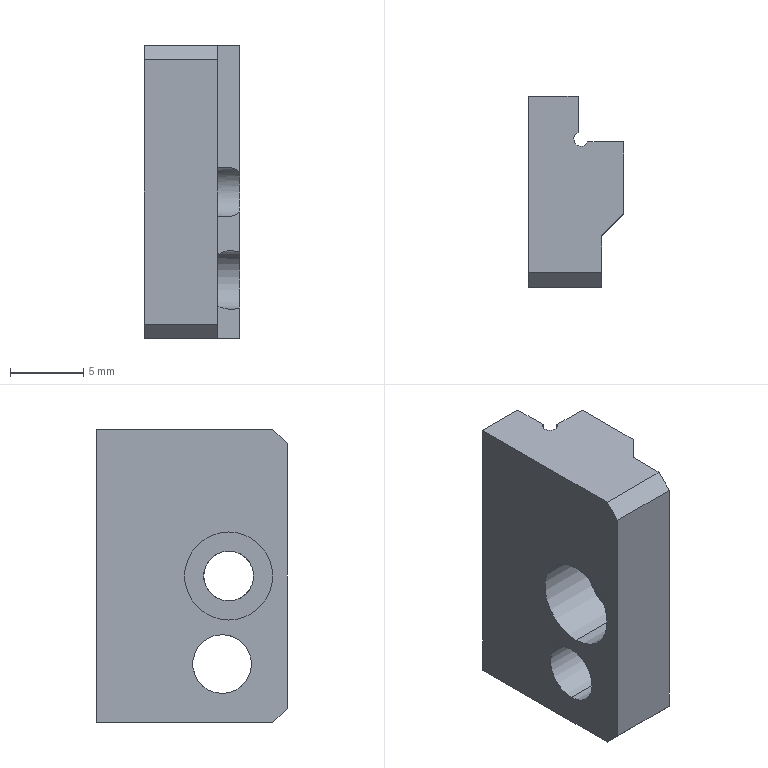Part | SolidWorks | features Cut 2, Chamfer 1, Extrusion 1, HoleWzd 1 | 1 solid | 23 faces | box 6.5 x 13 x 20 mm | volume 1157 mm3 | plane 15 | cylinder 8 | commonest cylinder face diameters 1 x2 3.4 x2 4 x2 6 x2
STEP:
#1=CARTESIAN_POINT('',(5.95,4.45,2.));
#2=VERTEX_POINT('',#1);
#3=CARTESIAN_POINT('',(5.,3.5,2.24));
#4=VERTEX_POINT('',#3);
#5=CARTESIAN_POINT('',(5.95,4.45,2.));
#6=CARTESIAN_POINT('',(5.617,4.117,2.));
#7=CARTESIAN_POINT('',(5.293,3.793,2.082));
#8=CARTESIAN_POINT('',(5.,3.5,2.24));
#9=(BOUNDED_CURVE()B_SPLINE_CURVE(3,(#5,#6,#7,#8),.UNSPECIFIED.,.F.,.F.)B_SPLINE_CURVE_WITH_KNOTS((4,4),(4.712,5.207),.UNSPECIFIED.)CURVE()GEOMETRIC_REPRESENTATION_ITEM()RATIONAL_B_SPLINE_CURVE((1.,0.9797,0.9797,1.))REPRESENTATION_ITEM(''));
#10=EDGE_CURVE('',#2,#4,#9,.T.);
#11=ORIENTED_EDGE('',*,*,#10,.F.);
#12=CARTESIAN_POINT('',(0.,4.45,2.));
#13=VERTEX_POINT('',#12);
#14=CARTESIAN_POINT('',(8.,4.45,2.));
#15=DIRECTION('',(-1.,0.,0.));
#16=VECTOR('',#15,1000.);
#17=LINE('',#14,#16);
#18=EDGE_CURVE('',#2,#13,#17,.T.);
#19=ORIENTED_EDGE('',*,*,#18,.T.);
#20=CARTESIAN_POINT('',(0.,4.45,6.));
#21=VERTEX_POINT('',#20);
#22=CARTESIAN_POINT('',(0.,4.45,4.));
#23=DIRECTION('',(-1.,0.,0.));
#24=DIRECTION('',(0.,0.,1.));
#25=AXIS2_PLACEMENT_3D('',#22,#23,#24);
#26=CIRCLE('',#25,2.);
#27=EDGE_CURVE('',#13,#21,#26,.T.);
#28=ORIENTED_EDGE('',*,*,#27,.T.);
#29=CARTESIAN_POINT('',(5.95,4.45,6.));
#30=VERTEX_POINT('',#29);
#31=CARTESIAN_POINT('',(8.,4.45,6.));
#32=DIRECTION('',(-1.,0.,0.));
#33=VECTOR('',#32,1000.);
#34=LINE('',#31,#33);
#35=EDGE_CURVE('',#30,#21,#34,.T.);
#36=ORIENTED_EDGE('',*,*,#35,.F.);
#37=CARTESIAN_POINT('',(5.,3.5,5.76));
#38=VERTEX_POINT('',#37);
#39=CARTESIAN_POINT('',(5.,3.5,5.76));
#40=CARTESIAN_POINT('',(5.293,3.793,5.918));
#41=CARTESIAN_POINT('',(5.617,4.117,6.));
#42=CARTESIAN_POINT('',(5.95,4.45,6.));
#43=(BOUNDED_CURVE()B_SPLINE_CURVE(3,(#39,#40,#41,#42),.UNSPECIFIED.,.F.,.T.)B_SPLINE_CURVE_WITH_KNOTS((4,4),(1.076,1.571),.UNSPECIFIED.)CURVE()GEOMETRIC_REPRESENTATION_ITEM()RATIONAL_B_SPLINE_CURVE((1.,0.9797,0.9797,1.))REPRESENTATION_ITEM(''));
#44=EDGE_CURVE('',#38,#30,#43,.T.);
#45=ORIENTED_EDGE('',*,*,#44,.F.);
#46=CARTESIAN_POINT('',(5.,4.45,4.));
#47=DIRECTION('',(-1.,0.,0.));
#48=DIRECTION('',(0.,0.,1.));
#49=AXIS2_PLACEMENT_3D('',#46,#47,#48);
#50=CIRCLE('',#49,2.);
#51=EDGE_CURVE('',#4,#38,#50,.T.);
#52=ORIENTED_EDGE('',*,*,#51,.F.);
#53=EDGE_LOOP('',(#11,#19,#28,#36,#45,#52));
#54=FACE_OUTER_BOUND('',#53,.T.);
#55=CARTESIAN_POINT('',(8.,4.45,4.));
#56=DIRECTION('',(-1.,0.,0.));
#57=DIRECTION('',(0.,0.,1.));
#58=AXIS2_PLACEMENT_3D('',#55,#56,#57);
#59=CYLINDRICAL_SURFACE('',#58,2.);
#60=ADVANCED_FACE('',(#54),#59,.F.);
#61=CARTESIAN_POINT('',(4.,4.,7.));
#62=VERTEX_POINT('',#61);
#63=CARTESIAN_POINT('',(4.,4.,13.));
#64=VERTEX_POINT('',#63);
#65=CARTESIAN_POINT('',(4.,4.,10.));
#66=DIRECTION('',(-1.,0.,0.));
#67=DIRECTION('',(0.,0.,1.));
#68=AXIS2_PLACEMENT_3D('',#65,#66,#67);
#69=CIRCLE('',#68,3.);
#70=EDGE_CURVE('',#62,#64,#69,.T.);
#71=ORIENTED_EDGE('',*,*,#70,.F.);
#72=CARTESIAN_POINT('',(0.,4.,7.));
#73=VERTEX_POINT('',#72);
#74=CARTESIAN_POINT('',(0.,4.,7.));
#75=DIRECTION('',(-1.,0.,0.));
#76=VECTOR('',#75,1000.);
#77=LINE('',#74,#76);
#78=EDGE_CURVE('',#62,#73,#77,.T.);
#79=ORIENTED_EDGE('',*,*,#78,.T.);
#80=CARTESIAN_POINT('',(0.,4.,13.));
#81=VERTEX_POINT('',#80);
#82=CARTESIAN_POINT('',(0.,4.,10.));
#83=DIRECTION('',(-1.,0.,0.));
#84=DIRECTION('',(0.,0.,1.));
#85=AXIS2_PLACEMENT_3D('',#82,#83,#84);
#86=CIRCLE('',#85,3.);
#87=EDGE_CURVE('',#73,#81,#86,.T.);
#88=ORIENTED_EDGE('',*,*,#87,.T.);
#89=CARTESIAN_POINT('',(0.,4.,13.));
#90=DIRECTION('',(-1.,0.,0.));
#91=VECTOR('',#90,1000.);
#92=LINE('',#89,#91);
#93=EDGE_CURVE('',#64,#81,#92,.T.);
#94=ORIENTED_EDGE('',*,*,#93,.F.);
#95=EDGE_LOOP('',(#71,#79,#88,#94));
#96=FACE_OUTER_BOUND('',#95,.T.);
#97=CARTESIAN_POINT('',(0.,4.,10.));
#98=DIRECTION('',(-1.,0.,0.));
#99=DIRECTION('',(0.,0.,1.));
#100=AXIS2_PLACEMENT_3D('',#97,#98,#99);
#101=CYLINDRICAL_SURFACE('',#100,3.);
#102=ADVANCED_FACE('',(#96),#101,.F.);
#103=CARTESIAN_POINT('',(5.5,4.,8.3));
#104=VERTEX_POINT('',#103);
#105=CARTESIAN_POINT('',(5.,3.5,8.375));
#106=VERTEX_POINT('',#105);
#107=CARTESIAN_POINT('',(5.5,4.,8.3));
#108=CARTESIAN_POINT('',(5.33,3.83,8.3));
#109=CARTESIAN_POINT('',(5.162,3.662,8.325));
#110=CARTESIAN_POINT('',(5.,3.5,8.375));
#111=(BOUNDED_CURVE()B_SPLINE_CURVE(3,(#107,#108,#109,#110),.UNSPECIFIED.,.F.,.F.)B_SPLINE_CURVE_WITH_KNOTS((4,4),(4.712,5.011),.UNSPECIFIED.)CURVE()GEOMETRIC_REPRESENTATION_ITEM()RATIONAL_B_SPLINE_CURVE((1.,0.9926,0.9926,1.))REPRESENTATION_ITEM(''));
#112=EDGE_CURVE('',#104,#106,#111,.T.);
#113=ORIENTED_EDGE('',*,*,#112,.F.);
#114=CARTESIAN_POINT('',(4.,4.,8.3));
#115=VERTEX_POINT('',#114);
#116=CARTESIAN_POINT('',(0.,4.,8.3));
#117=DIRECTION('',(-1.,0.,0.));
#118=VECTOR('',#117,1000.);
#119=LINE('',#116,#118);
#120=EDGE_CURVE('',#104,#115,#119,.T.);
#121=ORIENTED_EDGE('',*,*,#120,.T.);
#122=CARTESIAN_POINT('',(4.,4.,11.7));
#123=VERTEX_POINT('',#122);
#124=CARTESIAN_POINT('',(4.,4.,10.));
#125=DIRECTION('',(-1.,0.,0.));
#126=DIRECTION('',(0.,0.,1.));
#127=AXIS2_PLACEMENT_3D('',#124,#125,#126);
#128=CIRCLE('',#127,1.7);
#129=EDGE_CURVE('',#115,#123,#128,.T.);
#130=ORIENTED_EDGE('',*,*,#129,.T.);
#131=CARTESIAN_POINT('',(5.5,4.,11.7));
#132=VERTEX_POINT('',#131);
#133=CARTESIAN_POINT('',(0.,4.,11.7));
#134=DIRECTION('',(-1.,0.,0.));
#135=VECTOR('',#134,1000.);
#136=LINE('',#133,#135);
#137=EDGE_CURVE('',#132,#123,#136,.T.);
#138=ORIENTED_EDGE('',*,*,#137,.F.);
#139=CARTESIAN_POINT('',(5.,3.5,11.625));
#140=VERTEX_POINT('',#139);
#141=CARTESIAN_POINT('',(5.,3.5,11.625));
#142=CARTESIAN_POINT('',(5.162,3.662,11.675));
#143=CARTESIAN_POINT('',(5.33,3.83,11.7));
#144=CARTESIAN_POINT('',(5.5,4.,11.7));
#145=(BOUNDED_CURVE()B_SPLINE_CURVE(3,(#141,#142,#143,#144),.UNSPECIFIED.,.F.,.F.)B_SPLINE_CURVE_WITH_KNOTS((4,4),(1.272,1.571),.UNSPECIFIED.)CURVE()GEOMETRIC_REPRESENTATION_ITEM()RATIONAL_B_SPLINE_CURVE((1.,0.9926,0.9926,1.))REPRESENTATION_ITEM(''));
#146=EDGE_CURVE('',#140,#132,#145,.T.);
#147=ORIENTED_EDGE('',*,*,#146,.F.);
#148=CARTESIAN_POINT('',(5.,4.,10.));
#149=DIRECTION('',(-1.,0.,0.));
#150=DIRECTION('',(0.,0.,1.));
#151=AXIS2_PLACEMENT_3D('',#148,#149,#150);
#152=CIRCLE('',#151,1.7);
#153=EDGE_CURVE('',#106,#140,#152,.T.);
#154=ORIENTED_EDGE('',*,*,#153,.F.);
#155=EDGE_LOOP('',(#113,#121,#130,#138,#147,#154));
#156=FACE_OUTER_BOUND('',#155,.T.);
#157=CARTESIAN_POINT('',(0.,4.,10.));
#158=DIRECTION('',(-1.,0.,0.));
#159=DIRECTION('',(0.,0.,1.));
#160=AXIS2_PLACEMENT_3D('',#157,#158,#159);
#161=CYLINDRICAL_SURFACE('',#160,1.7);
#162=ADVANCED_FACE('',(#156),#161,.F.);
#163=CARTESIAN_POINT('',(3.1,10.1,20.));
#164=VERTEX_POINT('',#163);
#165=CARTESIAN_POINT('',(3.4,10.558,20.));
#166=VERTEX_POINT('',#165);
#167=CARTESIAN_POINT('',(3.6,10.1,20.));
#168=DIRECTION('',(0.,0.,-1.));
#169=DIRECTION('',(1.,0.,0.));
#170=AXIS2_PLACEMENT_3D('',#167,#168,#169);
#171=CIRCLE('',#170,0.5);
#172=EDGE_CURVE('',#164,#166,#171,.T.);
#173=ORIENTED_EDGE('',*,*,#172,.F.);
#174=CARTESIAN_POINT('',(3.1,10.1,0.));
#175=VERTEX_POINT('',#174);
#176=CARTESIAN_POINT('',(3.1,10.1,20.));
#177=DIRECTION('',(0.,0.,-1.));
#178=VECTOR('',#177,1000.);
#179=LINE('',#176,#178);
#180=EDGE_CURVE('',#164,#175,#179,.T.);
#181=ORIENTED_EDGE('',*,*,#180,.T.);
#182=CARTESIAN_POINT('',(3.4,10.558,0.));
#183=VERTEX_POINT('',#182);
#184=CARTESIAN_POINT('',(3.6,10.1,0.));
#185=DIRECTION('',(0.,0.,-1.));
#186=DIRECTION('',(1.,0.,0.));
#187=AXIS2_PLACEMENT_3D('',#184,#185,#186);
#188=CIRCLE('',#187,0.5);
#189=EDGE_CURVE('',#175,#183,#188,.T.);
#190=ORIENTED_EDGE('',*,*,#189,.T.);
#191=CARTESIAN_POINT('',(3.4,10.558,20.));
#192=DIRECTION('',(0.,0.,-1.));
#193=VECTOR('',#192,1000.);
#194=LINE('',#191,#193);
#195=EDGE_CURVE('',#166,#183,#194,.T.);
#196=ORIENTED_EDGE('',*,*,#195,.F.);
#197=EDGE_LOOP('',(#173,#181,#190,#196));
#198=FACE_OUTER_BOUND('',#197,.T.);
#199=CARTESIAN_POINT('',(3.6,10.1,20.));
#200=DIRECTION('',(0.,0.,-1.));
#201=DIRECTION('',(-1.,0.,0.));
#202=AXIS2_PLACEMENT_3D('',#199,#200,#201);
#203=CYLINDRICAL_SURFACE('',#202,0.5);
#204=ADVANCED_FACE('',(#198),#203,.F.);
#205=CARTESIAN_POINT('',(5.,3.5,-5.22));
#206=DIRECTION('',(0.,0.,1.));
#207=VECTOR('',#206,1000.);
#208=LINE('',#205,#207);
#209=EDGE_CURVE('',#38,#106,#208,.T.);
#210=ORIENTED_EDGE('',*,*,#209,.F.);
#211=ORIENTED_EDGE('',*,*,#44,.T.);
#212=CARTESIAN_POINT('',(6.5,5.,5.923));
#213=VERTEX_POINT('',#212);
#214=CARTESIAN_POINT('',(5.95,4.45,6.));
#215=CARTESIAN_POINT('',(6.136,4.636,6.));
#216=CARTESIAN_POINT('',(6.321,4.821,5.974));
#217=CARTESIAN_POINT('',(6.5,5.,5.923));
#218=(BOUNDED_CURVE()B_SPLINE_CURVE(3,(#214,#215,#216,#217),.UNSPECIFIED.,.F.,.F.)B_SPLINE_CURVE_WITH_KNOTS((4,4),(1.571,1.849),.UNSPECIFIED.)CURVE()GEOMETRIC_REPRESENTATION_ITEM()RATIONAL_B_SPLINE_CURVE((1.,0.9935,0.9935,1.))REPRESENTATION_ITEM(''));
#219=EDGE_CURVE('',#30,#213,#218,.T.);
#220=ORIENTED_EDGE('',*,*,#219,.T.);
#221=CARTESIAN_POINT('',(6.5,5.,8.625));
#222=VERTEX_POINT('',#221);
#223=CARTESIAN_POINT('',(6.5,5.,-5.22));
#224=DIRECTION('',(0.,0.,1.));
#225=VECTOR('',#224,1000.);
#226=LINE('',#223,#225);
#227=EDGE_CURVE('',#213,#222,#226,.T.);
#228=ORIENTED_EDGE('',*,*,#227,.T.);
#229=CARTESIAN_POINT('',(6.5,5.,8.625));
#230=CARTESIAN_POINT('',(6.207,4.707,8.412));
#231=CARTESIAN_POINT('',(5.862,4.362,8.3));
#232=CARTESIAN_POINT('',(5.5,4.,8.3));
#233=(BOUNDED_CURVE()B_SPLINE_CURVE(3,(#229,#230,#231,#232),.UNSPECIFIED.,.F.,.F.)B_SPLINE_CURVE_WITH_KNOTS((4,4),(4.084,4.712),.UNSPECIFIED.)CURVE()GEOMETRIC_REPRESENTATION_ITEM()RATIONAL_B_SPLINE_CURVE((1.,0.9673,0.9673,1.))REPRESENTATION_ITEM(''));
#234=EDGE_CURVE('',#222,#104,#233,.T.);
#235=ORIENTED_EDGE('',*,*,#234,.T.);
#236=ORIENTED_EDGE('',*,*,#112,.T.);
#237=EDGE_LOOP('',(#210,#211,#220,#228,#235,#236));
#238=FACE_OUTER_BOUND('',#237,.T.);
#239=CARTESIAN_POINT('',(6.5,5.,-5.22));
#240=DIRECTION('',(-0.7071,0.7071,0.));
#241=DIRECTION('',(-0.7071,-0.7071,0.));
#242=AXIS2_PLACEMENT_3D('',#239,#240,#241);
#243=PLANE('',#242);
#244=ADVANCED_FACE('',(#238),#243,.F.);
#245=CARTESIAN_POINT('',(5.,3.5,20.));
#246=VERTEX_POINT('',#245);
#247=CARTESIAN_POINT('',(5.,3.5,-5.22));
#248=DIRECTION('',(0.,0.,1.));
#249=VECTOR('',#248,1000.);
#250=LINE('',#247,#249);
#251=EDGE_CURVE('',#140,#246,#250,.T.);
#252=ORIENTED_EDGE('',*,*,#251,.F.);
#253=ORIENTED_EDGE('',*,*,#146,.T.);
#254=CARTESIAN_POINT('',(6.5,5.,11.375));
#255=VERTEX_POINT('',#254);
#256=CARTESIAN_POINT('',(5.5,4.,11.7));
#257=CARTESIAN_POINT('',(5.862,4.362,11.7));
#258=CARTESIAN_POINT('',(6.207,4.707,11.588));
#259=CARTESIAN_POINT('',(6.5,5.,11.375));
#260=(BOUNDED_CURVE()B_SPLINE_CURVE(3,(#256,#257,#258,#259),.UNSPECIFIED.,.F.,.F.)B_SPLINE_CURVE_WITH_KNOTS((4,4),(1.571,2.2),.UNSPECIFIED.)CURVE()GEOMETRIC_REPRESENTATION_ITEM()RATIONAL_B_SPLINE_CURVE((1.,0.9673,0.9673,1.))REPRESENTATION_ITEM(''));
#261=EDGE_CURVE('',#132,#255,#260,.T.);
#262=ORIENTED_EDGE('',*,*,#261,.T.);
#263=CARTESIAN_POINT('',(6.5,5.,20.));
#264=VERTEX_POINT('',#263);
#265=CARTESIAN_POINT('',(6.5,5.,-5.22));
#266=DIRECTION('',(0.,0.,1.));
#267=VECTOR('',#266,1000.);
#268=LINE('',#265,#267);
#269=EDGE_CURVE('',#255,#264,#268,.T.);
#270=ORIENTED_EDGE('',*,*,#269,.T.);
#271=CARTESIAN_POINT('',(6.5,5.,20.));
#272=DIRECTION('',(-0.7071,-0.7071,0.));
#273=VECTOR('',#272,1000.);
#274=LINE('',#271,#273);
#275=EDGE_CURVE('',#264,#246,#274,.T.);
#276=ORIENTED_EDGE('',*,*,#275,.T.);
#277=EDGE_LOOP('',(#252,#253,#262,#270,#276));
#278=FACE_OUTER_BOUND('',#277,.T.);
#279=CARTESIAN_POINT('',(6.5,5.,-5.22));
#280=DIRECTION('',(-0.7071,0.7071,0.));
#281=DIRECTION('',(-0.7071,-0.7071,0.));
#282=AXIS2_PLACEMENT_3D('',#279,#280,#281);
#283=PLANE('',#282);
#284=ADVANCED_FACE('',(#278),#283,.F.);
#285=CARTESIAN_POINT('',(5.,0.,1.));
#286=VERTEX_POINT('',#285);
#287=CARTESIAN_POINT('',(5.,0.,19.));
#288=VERTEX_POINT('',#287);
#289=CARTESIAN_POINT('',(5.,0.,-5.22));
#290=DIRECTION('',(0.,0.,1.));
#291=VECTOR('',#290,1000.);
#292=LINE('',#289,#291);
#293=EDGE_CURVE('',#286,#288,#292,.T.);
#294=ORIENTED_EDGE('',*,*,#293,.T.);
#295=CARTESIAN_POINT('',(0.,0.,19.));
#296=VERTEX_POINT('',#295);
#297=CARTESIAN_POINT('',(0.,0.,19.));
#298=DIRECTION('',(-1.,0.,0.));
#299=VECTOR('',#298,1000.);
#300=LINE('',#297,#299);
#301=EDGE_CURVE('',#288,#296,#300,.T.);
#302=ORIENTED_EDGE('',*,*,#301,.T.);
#303=CARTESIAN_POINT('',(0.,0.,1.));
#304=VERTEX_POINT('',#303);
#305=CARTESIAN_POINT('',(0.,0.,20.));
#306=DIRECTION('',(0.,0.,-1.));
#307=VECTOR('',#306,1000.);
#308=LINE('',#305,#307);
#309=EDGE_CURVE('',#296,#304,#308,.T.);
#310=ORIENTED_EDGE('',*,*,#309,.T.);
#311=CARTESIAN_POINT('',(6.5,0.,1.));
#312=DIRECTION('',(1.,0.,0.));
#313=VECTOR('',#312,1000.);
#314=LINE('',#311,#313);
#315=EDGE_CURVE('',#304,#286,#314,.T.);
#316=ORIENTED_EDGE('',*,*,#315,.T.);
#317=EDGE_LOOP('',(#294,#302,#310,#316));
#318=FACE_OUTER_BOUND('',#317,.T.);
#319=CARTESIAN_POINT('',(6.5,0.,20.));
#320=DIRECTION('',(0.,1.,0.));
#321=DIRECTION('',(-1.,0.,0.));
#322=AXIS2_PLACEMENT_3D('',#319,#320,#321);
#323=PLANE('',#322);
#324=ADVANCED_FACE('',(#318),#323,.F.);
#325=ORIENTED_EDGE('',*,*,#227,.F.);
#326=CARTESIAN_POINT('',(6.5,5.,2.077));
#327=VERTEX_POINT('',#326);
#328=CARTESIAN_POINT('',(6.5,4.45,4.));
#329=DIRECTION('',(-1.,0.,0.));
#330=DIRECTION('',(0.,-1.,0.));
#331=AXIS2_PLACEMENT_3D('',#328,#329,#330);
#332=CIRCLE('',#331,2.);
#333=EDGE_CURVE('',#213,#327,#332,.T.);
#334=ORIENTED_EDGE('',*,*,#333,.T.);
#335=CARTESIAN_POINT('',(6.5,5.,0.));
#336=VERTEX_POINT('',#335);
#337=CARTESIAN_POINT('',(6.5,5.,-5.22));
#338=DIRECTION('',(0.,0.,1.));
#339=VECTOR('',#338,1000.);
#340=LINE('',#337,#339);
#341=EDGE_CURVE('',#336,#327,#340,.T.);
#342=ORIENTED_EDGE('',*,*,#341,.F.);
#343=CARTESIAN_POINT('',(6.5,9.9,0.));
#344=VERTEX_POINT('',#343);
#345=CARTESIAN_POINT('',(6.5,9.9,0.));
#346=DIRECTION('',(0.,1.,0.));
#347=VECTOR('',#346,1000.);
#348=LINE('',#345,#347);
#349=EDGE_CURVE('',#336,#344,#348,.T.);
#350=ORIENTED_EDGE('',*,*,#349,.T.);
#351=CARTESIAN_POINT('',(6.5,9.9,20.));
#352=VERTEX_POINT('',#351);
#353=CARTESIAN_POINT('',(6.5,9.9,20.));
#354=DIRECTION('',(0.,0.,-1.));
#355=VECTOR('',#354,1000.);
#356=LINE('',#353,#355);
#357=EDGE_CURVE('',#352,#344,#356,.T.);
#358=ORIENTED_EDGE('',*,*,#357,.F.);
#359=CARTESIAN_POINT('',(6.5,9.9,20.));
#360=DIRECTION('',(0.,1.,0.));
#361=VECTOR('',#360,1000.);
#362=LINE('',#359,#361);
#363=EDGE_CURVE('',#264,#352,#362,.T.);
#364=ORIENTED_EDGE('',*,*,#363,.F.);
#365=ORIENTED_EDGE('',*,*,#269,.F.);
#366=CARTESIAN_POINT('',(6.5,4.,10.));
#367=DIRECTION('',(-1.,0.,0.));
#368=DIRECTION('',(0.,-1.,0.));
#369=AXIS2_PLACEMENT_3D('',#366,#367,#368);
#370=CIRCLE('',#369,1.7);
#371=EDGE_CURVE('',#255,#222,#370,.T.);
#372=ORIENTED_EDGE('',*,*,#371,.T.);
#373=EDGE_LOOP('',(#325,#334,#342,#350,#358,#364,#365,#372));
#374=FACE_OUTER_BOUND('',#373,.T.);
#375=CARTESIAN_POINT('',(6.5,9.9,20.));
#376=DIRECTION('',(-1.,0.,0.));
#377=DIRECTION('',(0.,-1.,0.));
#378=AXIS2_PLACEMENT_3D('',#375,#376,#377);
#379=PLANE('',#378);
#380=ADVANCED_FACE('',(#374),#379,.F.);
#381=CARTESIAN_POINT('',(4.058,9.9,0.));
#382=VERTEX_POINT('',#381);
#383=CARTESIAN_POINT('',(4.058,9.9,0.));
#384=DIRECTION('',(-1.,0.,0.));
#385=VECTOR('',#384,1000.);
#386=LINE('',#383,#385);
#387=EDGE_CURVE('',#344,#382,#386,.T.);
#388=ORIENTED_EDGE('',*,*,#387,.T.);
#389=CARTESIAN_POINT('',(4.058,9.9,20.));
#390=VERTEX_POINT('',#389);
#391=CARTESIAN_POINT('',(4.058,9.9,20.));
#392=DIRECTION('',(0.,0.,-1.));
#393=VECTOR('',#392,1000.);
#394=LINE('',#391,#393);
#395=EDGE_CURVE('',#390,#382,#394,.T.);
#396=ORIENTED_EDGE('',*,*,#395,.F.);
#397=CARTESIAN_POINT('',(4.058,9.9,20.));
#398=DIRECTION('',(-1.,0.,0.));
#399=VECTOR('',#398,1000.);
#400=LINE('',#397,#399);
#401=EDGE_CURVE('',#352,#390,#400,.T.);
#402=ORIENTED_EDGE('',*,*,#401,.F.);
#403=ORIENTED_EDGE('',*,*,#357,.T.);
#404=EDGE_LOOP('',(#388,#396,#402,#403));
#405=FACE_OUTER_BOUND('',#404,.T.);
#406=CARTESIAN_POINT('',(4.058,9.9,20.));
#407=DIRECTION('',(0.,-1.,0.));
#408=DIRECTION('',(1.,0.,0.));
#409=AXIS2_PLACEMENT_3D('',#406,#407,#408);
#410=PLANE('',#409);
#411=ADVANCED_FACE('',(#405),#410,.F.);
#412=ORIENTED_EDGE('',*,*,#180,.F.);
#413=CARTESIAN_POINT('',(3.6,10.1,20.));
#414=DIRECTION('',(0.,0.,-1.));
#415=DIRECTION('',(1.,0.,0.));
#416=AXIS2_PLACEMENT_3D('',#413,#414,#415);
#417=CIRCLE('',#416,0.5);
#418=EDGE_CURVE('',#390,#164,#417,.T.);
#419=ORIENTED_EDGE('',*,*,#418,.F.);
#420=ORIENTED_EDGE('',*,*,#395,.T.);
#421=CARTESIAN_POINT('',(3.6,10.1,0.));
#422=DIRECTION('',(0.,0.,-1.));
#423=DIRECTION('',(1.,0.,0.));
#424=AXIS2_PLACEMENT_3D('',#421,#422,#423);
#425=CIRCLE('',#424,0.5);
#426=EDGE_CURVE('',#382,#175,#425,.T.);
#427=ORIENTED_EDGE('',*,*,#426,.T.);
#428=EDGE_LOOP('',(#412,#419,#420,#427));
#429=FACE_OUTER_BOUND('',#428,.T.);
#430=CARTESIAN_POINT('',(3.6,10.1,20.));
#431=DIRECTION('',(0.,0.,-1.));
#432=DIRECTION('',(-1.,0.,0.));
#433=AXIS2_PLACEMENT_3D('',#430,#431,#432);
#434=CYLINDRICAL_SURFACE('',#433,0.5);
#435=ADVANCED_FACE('',(#429),#434,.F.);
#436=CARTESIAN_POINT('',(3.4,13.,0.));
#437=VERTEX_POINT('',#436);
#438=CARTESIAN_POINT('',(3.4,13.,0.));
#439=DIRECTION('',(0.,1.,0.));
#440=VECTOR('',#439,1000.);
#441=LINE('',#438,#440);
#442=EDGE_CURVE('',#183,#437,#441,.T.);
#443=ORIENTED_EDGE('',*,*,#442,.T.);
#444=CARTESIAN_POINT('',(3.4,13.,20.));
#445=VERTEX_POINT('',#444);
#446=CARTESIAN_POINT('',(3.4,13.,20.));
#447=DIRECTION('',(0.,0.,-1.));
#448=VECTOR('',#447,1000.);
#449=LINE('',#446,#448);
#450=EDGE_CURVE('',#445,#437,#449,.T.);
#451=ORIENTED_EDGE('',*,*,#450,.F.);
#452=CARTESIAN_POINT('',(3.4,13.,20.));
#453=DIRECTION('',(0.,1.,0.));
#454=VECTOR('',#453,1000.);
#455=LINE('',#452,#454);
#456=EDGE_CURVE('',#166,#445,#455,.T.);
#457=ORIENTED_EDGE('',*,*,#456,.F.);
#458=ORIENTED_EDGE('',*,*,#195,.T.);
#459=EDGE_LOOP('',(#443,#451,#457,#458));
#460=FACE_OUTER_BOUND('',#459,.T.);
#461=CARTESIAN_POINT('',(3.4,13.,20.));
#462=DIRECTION('',(-1.,0.,0.));
#463=DIRECTION('',(0.,-1.,0.));
#464=AXIS2_PLACEMENT_3D('',#461,#462,#463);
#465=PLANE('',#464);
#466=ADVANCED_FACE('',(#460),#465,.F.);
#467=CARTESIAN_POINT('',(0.,13.,0.));
#468=VERTEX_POINT('',#467);
#469=CARTESIAN_POINT('',(0.,13.,0.));
#470=DIRECTION('',(-1.,0.,0.));
#471=VECTOR('',#470,1000.);
#472=LINE('',#469,#471);
#473=EDGE_CURVE('',#437,#468,#472,.T.);
#474=ORIENTED_EDGE('',*,*,#473,.T.);
#475=CARTESIAN_POINT('',(0.,13.,20.));
#476=VERTEX_POINT('',#475);
#477=CARTESIAN_POINT('',(0.,13.,20.));
#478=DIRECTION('',(0.,0.,-1.));
#479=VECTOR('',#478,1000.);
#480=LINE('',#477,#479);
#481=EDGE_CURVE('',#476,#468,#480,.T.);
#482=ORIENTED_EDGE('',*,*,#481,.F.);
#483=CARTESIAN_POINT('',(0.,13.,20.));
#484=DIRECTION('',(-1.,0.,0.));
#485=VECTOR('',#484,1000.);
#486=LINE('',#483,#485);
#487=EDGE_CURVE('',#445,#476,#486,.T.);
#488=ORIENTED_EDGE('',*,*,#487,.F.);
#489=ORIENTED_EDGE('',*,*,#450,.T.);
#490=EDGE_LOOP('',(#474,#482,#488,#489));
#491=FACE_OUTER_BOUND('',#490,.T.);
#492=CARTESIAN_POINT('',(0.,13.,20.));
#493=DIRECTION('',(0.,-1.,0.));
#494=DIRECTION('',(0.,0.,-1.));
#495=AXIS2_PLACEMENT_3D('',#492,#493,#494);
#496=PLANE('',#495);
#497=ADVANCED_FACE('',(#491),#496,.F.);
#498=CARTESIAN_POINT('',(0.,4.45,4.));
#499=DIRECTION('',(-1.,0.,0.));
#500=DIRECTION('',(0.,0.,1.));
#501=AXIS2_PLACEMENT_3D('',#498,#499,#500);
#502=CIRCLE('',#501,2.);
#503=EDGE_CURVE('',#21,#13,#502,.T.);
#504=ORIENTED_EDGE('',*,*,#503,.F.);
#505=ORIENTED_EDGE('',*,*,#27,.F.);
#506=EDGE_LOOP('',(#504,#505));
#507=FACE_BOUND('',#506,.T.);
#508=CARTESIAN_POINT('',(0.,4.,10.));
#509=DIRECTION('',(-1.,0.,0.));
#510=DIRECTION('',(0.,0.,1.));
#511=AXIS2_PLACEMENT_3D('',#508,#509,#510);
#512=CIRCLE('',#511,3.);
#513=EDGE_CURVE('',#81,#73,#512,.T.);
#514=ORIENTED_EDGE('',*,*,#513,.F.);
#515=ORIENTED_EDGE('',*,*,#87,.F.);
#516=EDGE_LOOP('',(#514,#515));
#517=FACE_BOUND('',#516,.T.);
#518=ORIENTED_EDGE('',*,*,#309,.F.);
#519=CARTESIAN_POINT('',(0.,1.,20.));
#520=VERTEX_POINT('',#519);
#521=CARTESIAN_POINT('',(0.,1.,20.));
#522=DIRECTION('',(0.,0.7071,0.7071));
#523=VECTOR('',#522,1000.);
#524=LINE('',#521,#523);
#525=EDGE_CURVE('',#296,#520,#524,.T.);
#526=ORIENTED_EDGE('',*,*,#525,.T.);
#527=CARTESIAN_POINT('',(0.,0.,20.));
#528=DIRECTION('',(0.,-1.,0.));
#529=VECTOR('',#528,1000.);
#530=LINE('',#527,#529);
#531=EDGE_CURVE('',#476,#520,#530,.T.);
#532=ORIENTED_EDGE('',*,*,#531,.F.);
#533=ORIENTED_EDGE('',*,*,#481,.T.);
#534=CARTESIAN_POINT('',(0.,1.,0.));
#535=VERTEX_POINT('',#534);
#536=CARTESIAN_POINT('',(0.,0.,0.));
#537=DIRECTION('',(0.,-1.,0.));
#538=VECTOR('',#537,1000.);
#539=LINE('',#536,#538);
#540=EDGE_CURVE('',#468,#535,#539,.T.);
#541=ORIENTED_EDGE('',*,*,#540,.T.);
#542=CARTESIAN_POINT('',(0.,0.,1.));
#543=DIRECTION('',(0.,-0.7071,0.7071));
#544=VECTOR('',#543,1000.);
#545=LINE('',#542,#544);
#546=EDGE_CURVE('',#535,#304,#545,.T.);
#547=ORIENTED_EDGE('',*,*,#546,.T.);
#548=EDGE_LOOP('',(#518,#526,#532,#533,#541,#547));
#549=FACE_OUTER_BOUND('',#548,.T.);
#550=CARTESIAN_POINT('',(0.,0.,20.));
#551=DIRECTION('',(1.,0.,0.));
#552=DIRECTION('',(0.,0.,-1.));
#553=AXIS2_PLACEMENT_3D('',#550,#551,#552);
#554=PLANE('',#553);
#555=ADVANCED_FACE('',(#507,#517,#549),#554,.F.);
#556=ORIENTED_EDGE('',*,*,#531,.T.);
#557=CARTESIAN_POINT('',(5.,1.,20.));
#558=VERTEX_POINT('',#557);
#559=CARTESIAN_POINT('',(5.,1.,20.));
#560=DIRECTION('',(1.,0.,0.));
#561=VECTOR('',#560,1000.);
#562=LINE('',#559,#561);
#563=EDGE_CURVE('',#520,#558,#562,.T.);
#564=ORIENTED_EDGE('',*,*,#563,.T.);
#565=CARTESIAN_POINT('',(5.,3.5,20.));
#566=DIRECTION('',(0.,-1.,0.));
#567=VECTOR('',#566,1000.);
#568=LINE('',#565,#567);
#569=EDGE_CURVE('',#246,#558,#568,.T.);
#570=ORIENTED_EDGE('',*,*,#569,.F.);
#571=ORIENTED_EDGE('',*,*,#275,.F.);
#572=ORIENTED_EDGE('',*,*,#363,.T.);
#573=ORIENTED_EDGE('',*,*,#401,.T.);
#574=ORIENTED_EDGE('',*,*,#418,.T.);
#575=ORIENTED_EDGE('',*,*,#172,.T.);
#576=ORIENTED_EDGE('',*,*,#456,.T.);
#577=ORIENTED_EDGE('',*,*,#487,.T.);
#578=EDGE_LOOP('',(#556,#564,#570,#571,#572,#573,#574,#575,#576,#577));
#579=FACE_OUTER_BOUND('',#578,.T.);
#580=CARTESIAN_POINT('',(3.6,10.1,20.));
#581=DIRECTION('',(0.,0.,1.));
#582=DIRECTION('',(1.,0.,0.));
#583=AXIS2_PLACEMENT_3D('',#580,#581,#582);
#584=PLANE('',#583);
#585=ADVANCED_FACE('',(#579),#584,.T.);
#586=CARTESIAN_POINT('',(5.,1.,0.));
#587=VERTEX_POINT('',#586);
#588=CARTESIAN_POINT('',(5.,3.5,0.));
#589=VERTEX_POINT('',#588);
#590=CARTESIAN_POINT('',(5.,3.5,0.));
#591=DIRECTION('',(0.,1.,0.));
#592=VECTOR('',#591,1000.);
#593=LINE('',#590,#592);
#594=EDGE_CURVE('',#587,#589,#593,.T.);
#595=ORIENTED_EDGE('',*,*,#594,.F.);
#596=CARTESIAN_POINT('',(3.6,1.,0.));
#597=DIRECTION('',(-1.,0.,0.));
#598=VECTOR('',#597,1000.);
#599=LINE('',#596,#598);
#600=EDGE_CURVE('',#587,#535,#599,.T.);
#601=ORIENTED_EDGE('',*,*,#600,.T.);
#602=ORIENTED_EDGE('',*,*,#540,.F.);
#603=ORIENTED_EDGE('',*,*,#473,.F.);
#604=ORIENTED_EDGE('',*,*,#442,.F.);
#605=ORIENTED_EDGE('',*,*,#189,.F.);
#606=ORIENTED_EDGE('',*,*,#426,.F.);
#607=ORIENTED_EDGE('',*,*,#387,.F.);
#608=ORIENTED_EDGE('',*,*,#349,.F.);
#609=CARTESIAN_POINT('',(6.5,5.,0.));
#610=DIRECTION('',(0.7071,0.7071,0.));
#611=VECTOR('',#610,1000.);
#612=LINE('',#609,#611);
#613=EDGE_CURVE('',#589,#336,#612,.T.);
#614=ORIENTED_EDGE('',*,*,#613,.F.);
#615=EDGE_LOOP('',(#595,#601,#602,#603,#604,#605,#606,#607,#608,#614));
#616=FACE_OUTER_BOUND('',#615,.T.);
#617=CARTESIAN_POINT('',(3.6,10.1,0.));
#618=DIRECTION('',(0.,0.,1.));
#619=DIRECTION('',(1.,0.,0.));
#620=AXIS2_PLACEMENT_3D('',#617,#618,#619);
#621=PLANE('',#620);
#622=ADVANCED_FACE('',(#616),#621,.F.);
#623=CARTESIAN_POINT('',(5.,3.5,-5.22));
#624=DIRECTION('',(0.,0.,1.));
#625=VECTOR('',#624,1000.);
#626=LINE('',#623,#625);
#627=EDGE_CURVE('',#589,#4,#626,.T.);
#628=ORIENTED_EDGE('',*,*,#627,.T.);
#629=ORIENTED_EDGE('',*,*,#51,.T.);
#630=ORIENTED_EDGE('',*,*,#209,.T.);
#631=ORIENTED_EDGE('',*,*,#153,.T.);
#632=ORIENTED_EDGE('',*,*,#251,.T.);
#633=ORIENTED_EDGE('',*,*,#569,.T.);
#634=CARTESIAN_POINT('',(5.,1.,20.));
#635=DIRECTION('',(0.,-0.7071,-0.7071));
#636=VECTOR('',#635,1000.);
#637=LINE('',#634,#636);
#638=EDGE_CURVE('',#558,#288,#637,.T.);
#639=ORIENTED_EDGE('',*,*,#638,.T.);
#640=ORIENTED_EDGE('',*,*,#293,.F.);
#641=CARTESIAN_POINT('',(5.,0.,1.));
#642=DIRECTION('',(0.,0.7071,-0.7071));
#643=VECTOR('',#642,1000.);
#644=LINE('',#641,#643);
#645=EDGE_CURVE('',#286,#587,#644,.T.);
#646=ORIENTED_EDGE('',*,*,#645,.T.);
#647=ORIENTED_EDGE('',*,*,#594,.T.);
#648=EDGE_LOOP('',(#628,#629,#630,#631,#632,#633,#639,#640,#646,#647));
#649=FACE_OUTER_BOUND('',#648,.T.);
#650=CARTESIAN_POINT('',(5.,3.5,-5.22));
#651=DIRECTION('',(-1.,0.,0.));
#652=DIRECTION('',(0.,0.,1.));
#653=AXIS2_PLACEMENT_3D('',#650,#651,#652);
#654=PLANE('',#653);
#655=ADVANCED_FACE('',(#649),#654,.F.);
#656=ORIENTED_EDGE('',*,*,#341,.T.);
#657=CARTESIAN_POINT('',(6.5,5.,2.077));
#658=CARTESIAN_POINT('',(6.321,4.821,2.026));
#659=CARTESIAN_POINT('',(6.136,4.636,2.));
#660=CARTESIAN_POINT('',(5.95,4.45,2.));
#661=(BOUNDED_CURVE()B_SPLINE_CURVE(3,(#657,#658,#659,#660),.UNSPECIFIED.,.F.,.F.)B_SPLINE_CURVE_WITH_KNOTS((4,4),(4.434,4.712),.UNSPECIFIED.)CURVE()GEOMETRIC_REPRESENTATION_ITEM()RATIONAL_B_SPLINE_CURVE((1.,0.9935,0.9935,1.))REPRESENTATION_ITEM(''));
#662=EDGE_CURVE('',#327,#2,#661,.T.);
#663=ORIENTED_EDGE('',*,*,#662,.T.);
#664=ORIENTED_EDGE('',*,*,#10,.T.);
#665=ORIENTED_EDGE('',*,*,#627,.F.);
#666=ORIENTED_EDGE('',*,*,#613,.T.);
#667=EDGE_LOOP('',(#656,#663,#664,#665,#666));
#668=FACE_OUTER_BOUND('',#667,.T.);
#669=CARTESIAN_POINT('',(6.5,5.,-5.22));
#670=DIRECTION('',(-0.7071,0.7071,0.));
#671=DIRECTION('',(-0.7071,-0.7071,0.));
#672=AXIS2_PLACEMENT_3D('',#669,#670,#671);
#673=PLANE('',#672);
#674=ADVANCED_FACE('',(#668),#673,.F.);
#675=ORIENTED_EDGE('',*,*,#120,.F.);
#676=ORIENTED_EDGE('',*,*,#234,.F.);
#677=ORIENTED_EDGE('',*,*,#371,.F.);
#678=ORIENTED_EDGE('',*,*,#261,.F.);
#679=ORIENTED_EDGE('',*,*,#137,.T.);
#680=CARTESIAN_POINT('',(4.,4.,10.));
#681=DIRECTION('',(-1.,0.,0.));
#682=DIRECTION('',(0.,0.,1.));
#683=AXIS2_PLACEMENT_3D('',#680,#681,#682);
#684=CIRCLE('',#683,1.7);
#685=EDGE_CURVE('',#123,#115,#684,.T.);
#686=ORIENTED_EDGE('',*,*,#685,.T.);
#687=EDGE_LOOP('',(#675,#676,#677,#678,#679,#686));
#688=FACE_OUTER_BOUND('',#687,.T.);
#689=CARTESIAN_POINT('',(0.,4.,10.));
#690=DIRECTION('',(-1.,0.,0.));
#691=DIRECTION('',(0.,0.,1.));
#692=AXIS2_PLACEMENT_3D('',#689,#690,#691);
#693=CYLINDRICAL_SURFACE('',#692,1.7);
#694=ADVANCED_FACE('',(#688),#693,.F.);
#695=ORIENTED_EDGE('',*,*,#685,.F.);
#696=ORIENTED_EDGE('',*,*,#129,.F.);
#697=EDGE_LOOP('',(#695,#696));
#698=FACE_BOUND('',#697,.T.);
#699=CARTESIAN_POINT('',(4.,4.,10.));
#700=DIRECTION('',(-1.,0.,0.));
#701=DIRECTION('',(0.,0.,1.));
#702=AXIS2_PLACEMENT_3D('',#699,#700,#701);
#703=CIRCLE('',#702,3.);
#704=EDGE_CURVE('',#64,#62,#703,.T.);
#705=ORIENTED_EDGE('',*,*,#704,.T.);
#706=ORIENTED_EDGE('',*,*,#70,.T.);
#707=EDGE_LOOP('',(#705,#706));
#708=FACE_OUTER_BOUND('',#707,.T.);
#709=CARTESIAN_POINT('',(4.,5.7,10.));
#710=DIRECTION('',(1.,0.,0.));
#711=DIRECTION('',(0.,0.,-1.));
#712=AXIS2_PLACEMENT_3D('',#709,#710,#711);
#713=PLANE('',#712);
#714=ADVANCED_FACE('',(#698,#708),#713,.F.);
#715=ORIENTED_EDGE('',*,*,#78,.F.);
#716=ORIENTED_EDGE('',*,*,#704,.F.);
#717=ORIENTED_EDGE('',*,*,#93,.T.);
#718=ORIENTED_EDGE('',*,*,#513,.T.);
#719=EDGE_LOOP('',(#715,#716,#717,#718));
#720=FACE_OUTER_BOUND('',#719,.T.);
#721=CARTESIAN_POINT('',(0.,4.,10.));
#722=DIRECTION('',(-1.,0.,0.));
#723=DIRECTION('',(0.,0.,1.));
#724=AXIS2_PLACEMENT_3D('',#721,#722,#723);
#725=CYLINDRICAL_SURFACE('',#724,3.);
#726=ADVANCED_FACE('',(#720),#725,.F.);
#727=ORIENTED_EDGE('',*,*,#525,.F.);
#728=ORIENTED_EDGE('',*,*,#301,.F.);
#729=ORIENTED_EDGE('',*,*,#638,.F.);
#730=ORIENTED_EDGE('',*,*,#563,.F.);
#731=EDGE_LOOP('',(#727,#728,#729,#730));
#732=FACE_OUTER_BOUND('',#731,.T.);
#733=CARTESIAN_POINT('',(3.6,1.,20.));
#734=DIRECTION('',(0.,-0.7071,0.7071));
#735=DIRECTION('',(-1.,0.,0.));
#736=AXIS2_PLACEMENT_3D('',#733,#734,#735);
#737=PLANE('',#736);
#738=ADVANCED_FACE('',(#732),#737,.T.);
#739=ORIENTED_EDGE('',*,*,#546,.F.);
#740=ORIENTED_EDGE('',*,*,#600,.F.);
#741=ORIENTED_EDGE('',*,*,#645,.F.);
#742=ORIENTED_EDGE('',*,*,#315,.F.);
#743=EDGE_LOOP('',(#739,#740,#741,#742));
#744=FACE_OUTER_BOUND('',#743,.T.);
#745=CARTESIAN_POINT('',(6.5,0.,1.));
#746=DIRECTION('',(0.,0.7071,0.7071));
#747=DIRECTION('',(1.,0.,0.));
#748=AXIS2_PLACEMENT_3D('',#745,#746,#747);
#749=PLANE('',#748);
#750=ADVANCED_FACE('',(#744),#749,.F.);
#751=ORIENTED_EDGE('',*,*,#18,.F.);
#752=ORIENTED_EDGE('',*,*,#662,.F.);
#753=ORIENTED_EDGE('',*,*,#333,.F.);
#754=ORIENTED_EDGE('',*,*,#219,.F.);
#755=ORIENTED_EDGE('',*,*,#35,.T.);
#756=ORIENTED_EDGE('',*,*,#503,.T.);
#757=EDGE_LOOP('',(#751,#752,#753,#754,#755,#756));
#758=FACE_OUTER_BOUND('',#757,.T.);
#759=CARTESIAN_POINT('',(8.,4.45,4.));
#760=DIRECTION('',(-1.,0.,0.));
#761=DIRECTION('',(0.,0.,1.));
#762=AXIS2_PLACEMENT_3D('',#759,#760,#761);
#763=CYLINDRICAL_SURFACE('',#762,2.);
#764=ADVANCED_FACE('',(#758),#763,.F.);
#765=CLOSED_SHELL('',(#60,#102,#162,#204,#244,#284,#324,#380,#411,#435,#466,#497,#555,#585,#622,#655,#674,#694,#714,#726,#738,#750,#764));
#766=MANIFOLD_SOLID_BREP('',#765);
#767=CARTESIAN_POINT('',(0.,0.,0.));
#768=DIRECTION('',(0.,0.,1.));
#769=DIRECTION('',(1.,0.,0.));
#770=AXIS2_PLACEMENT_3D('',#767,#768,#769);
#771=(LENGTH_UNIT()NAMED_UNIT(*)SI_UNIT(.MILLI.,.METRE.));
#772=UNCERTAINTY_MEASURE_WITH_UNIT(LENGTH_MEASURE(0.00001),#771,'','');
#773=(NAMED_UNIT(*)PLANE_ANGLE_UNIT()SI_UNIT($,.RADIAN.));
#774=(NAMED_UNIT(*)SI_UNIT($,.STERADIAN.)SOLID_ANGLE_UNIT());
#775=(GEOMETRIC_REPRESENTATION_CONTEXT(3)GLOBAL_UNCERTAINTY_ASSIGNED_CONTEXT((#772))GLOBAL_UNIT_ASSIGNED_CONTEXT((#771,#773,#774))REPRESENTATION_CONTEXT('',''));
#776=ADVANCED_BREP_SHAPE_REPRESENTATION('',(#766,#770),#775);